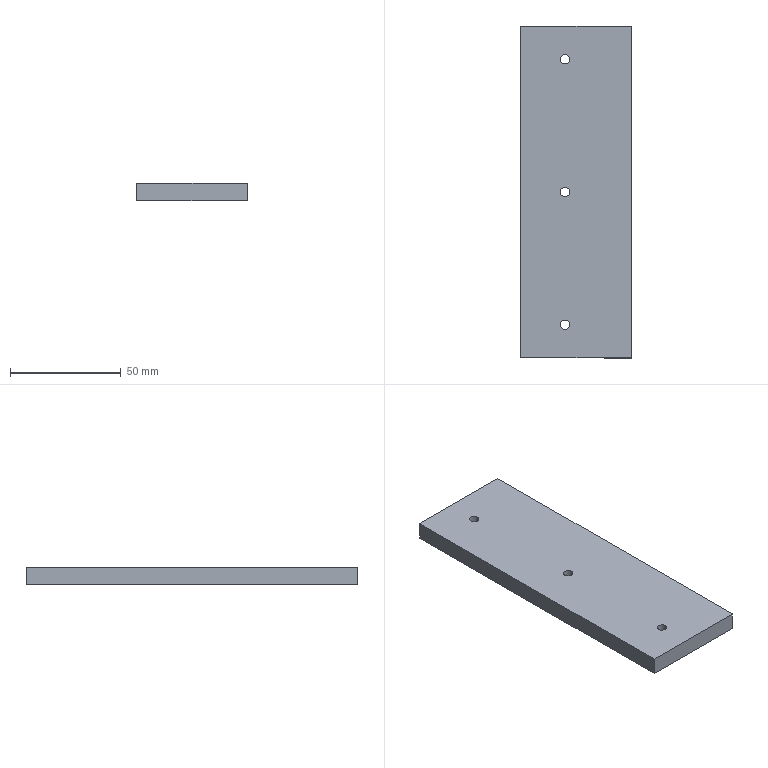Part | SolidWorks | features Chamfer 1, Extrusion 1, HoleWzd 1 | 1 solid | 12 faces | box 50 x 150 x 8 mm | volume 59667 mm3 | cylinder 6 | plane 6 | commonest cylinder face diameters 4.2 x6
STEP:
#1=CARTESIAN_POINT('',(-7.1,60.,-4.));
#2=VERTEX_POINT('',#1);
#3=CARTESIAN_POINT('',(-2.9,60.,-4.));
#4=VERTEX_POINT('',#3);
#5=CARTESIAN_POINT('',(-5.,60.,-4.));
#6=DIRECTION('',(0.,0.,1.));
#7=DIRECTION('',(1.,0.,0.));
#8=AXIS2_PLACEMENT_3D('',#5,#6,#7);
#9=CIRCLE('',#8,2.1);
#10=EDGE_CURVE('',#2,#4,#9,.T.);
#11=ORIENTED_EDGE('',*,*,#10,.F.);
#12=CARTESIAN_POINT('',(-7.1,60.,4.));
#13=VERTEX_POINT('',#12);
#14=CARTESIAN_POINT('',(-7.1,60.,4.));
#15=DIRECTION('',(0.,0.,1.));
#16=VECTOR('',#15,1000.);
#17=LINE('',#14,#16);
#18=EDGE_CURVE('',#2,#13,#17,.T.);
#19=ORIENTED_EDGE('',*,*,#18,.T.);
#20=CARTESIAN_POINT('',(-2.9,60.,4.));
#21=VERTEX_POINT('',#20);
#22=CARTESIAN_POINT('',(-5.,60.,4.));
#23=DIRECTION('',(0.,0.,1.));
#24=DIRECTION('',(1.,0.,0.));
#25=AXIS2_PLACEMENT_3D('',#22,#23,#24);
#26=CIRCLE('',#25,2.1);
#27=EDGE_CURVE('',#13,#21,#26,.T.);
#28=ORIENTED_EDGE('',*,*,#27,.T.);
#29=CARTESIAN_POINT('',(-2.9,60.,4.));
#30=DIRECTION('',(0.,0.,1.));
#31=VECTOR('',#30,1000.);
#32=LINE('',#29,#31);
#33=EDGE_CURVE('',#4,#21,#32,.T.);
#34=ORIENTED_EDGE('',*,*,#33,.F.);
#35=EDGE_LOOP('',(#11,#19,#28,#34));
#36=FACE_OUTER_BOUND('',#35,.T.);
#37=CARTESIAN_POINT('',(-5.,60.,4.));
#38=DIRECTION('',(0.,0.,1.));
#39=DIRECTION('',(1.,0.,0.));
#40=AXIS2_PLACEMENT_3D('',#37,#38,#39);
#41=CYLINDRICAL_SURFACE('',#40,2.1);
#42=ADVANCED_FACE('',(#36),#41,.F.);
#43=CARTESIAN_POINT('',(-7.1,-60.,-4.));
#44=VERTEX_POINT('',#43);
#45=CARTESIAN_POINT('',(-2.9,-60.,-4.));
#46=VERTEX_POINT('',#45);
#47=CARTESIAN_POINT('',(-5.,-60.,-4.));
#48=DIRECTION('',(0.,0.,1.));
#49=DIRECTION('',(1.,0.,0.));
#50=AXIS2_PLACEMENT_3D('',#47,#48,#49);
#51=CIRCLE('',#50,2.1);
#52=EDGE_CURVE('',#44,#46,#51,.T.);
#53=ORIENTED_EDGE('',*,*,#52,.F.);
#54=CARTESIAN_POINT('',(-7.1,-60.,4.));
#55=VERTEX_POINT('',#54);
#56=CARTESIAN_POINT('',(-7.1,-60.,4.));
#57=DIRECTION('',(0.,0.,1.));
#58=VECTOR('',#57,1000.);
#59=LINE('',#56,#58);
#60=EDGE_CURVE('',#44,#55,#59,.T.);
#61=ORIENTED_EDGE('',*,*,#60,.T.);
#62=CARTESIAN_POINT('',(-2.9,-60.,4.));
#63=VERTEX_POINT('',#62);
#64=CARTESIAN_POINT('',(-5.,-60.,4.));
#65=DIRECTION('',(0.,0.,1.));
#66=DIRECTION('',(1.,0.,0.));
#67=AXIS2_PLACEMENT_3D('',#64,#65,#66);
#68=CIRCLE('',#67,2.1);
#69=EDGE_CURVE('',#55,#63,#68,.T.);
#70=ORIENTED_EDGE('',*,*,#69,.T.);
#71=CARTESIAN_POINT('',(-2.9,-60.,4.));
#72=DIRECTION('',(0.,0.,1.));
#73=VECTOR('',#72,1000.);
#74=LINE('',#71,#73);
#75=EDGE_CURVE('',#46,#63,#74,.T.);
#76=ORIENTED_EDGE('',*,*,#75,.F.);
#77=EDGE_LOOP('',(#53,#61,#70,#76));
#78=FACE_OUTER_BOUND('',#77,.T.);
#79=CARTESIAN_POINT('',(-5.,-60.,4.));
#80=DIRECTION('',(0.,0.,1.));
#81=DIRECTION('',(1.,0.,0.));
#82=AXIS2_PLACEMENT_3D('',#79,#80,#81);
#83=CYLINDRICAL_SURFACE('',#82,2.1);
#84=ADVANCED_FACE('',(#78),#83,.F.);
#85=CARTESIAN_POINT('',(-7.1,0.,-4.));
#86=VERTEX_POINT('',#85);
#87=CARTESIAN_POINT('',(-2.9,0.,-4.));
#88=VERTEX_POINT('',#87);
#89=CARTESIAN_POINT('',(-5.,0.,-4.));
#90=DIRECTION('',(0.,0.,1.));
#91=DIRECTION('',(1.,0.,0.));
#92=AXIS2_PLACEMENT_3D('',#89,#90,#91);
#93=CIRCLE('',#92,2.1);
#94=EDGE_CURVE('',#86,#88,#93,.T.);
#95=ORIENTED_EDGE('',*,*,#94,.F.);
#96=CARTESIAN_POINT('',(-7.1,0.,4.));
#97=VERTEX_POINT('',#96);
#98=CARTESIAN_POINT('',(-7.1,0.,4.));
#99=DIRECTION('',(0.,0.,1.));
#100=VECTOR('',#99,1000.);
#101=LINE('',#98,#100);
#102=EDGE_CURVE('',#86,#97,#101,.T.);
#103=ORIENTED_EDGE('',*,*,#102,.T.);
#104=CARTESIAN_POINT('',(-2.9,0.,4.));
#105=VERTEX_POINT('',#104);
#106=CARTESIAN_POINT('',(-5.,0.,4.));
#107=DIRECTION('',(0.,0.,1.));
#108=DIRECTION('',(1.,0.,0.));
#109=AXIS2_PLACEMENT_3D('',#106,#107,#108);
#110=CIRCLE('',#109,2.1);
#111=EDGE_CURVE('',#97,#105,#110,.T.);
#112=ORIENTED_EDGE('',*,*,#111,.T.);
#113=CARTESIAN_POINT('',(-2.9,0.,4.));
#114=DIRECTION('',(0.,0.,1.));
#115=VECTOR('',#114,1000.);
#116=LINE('',#113,#115);
#117=EDGE_CURVE('',#88,#105,#116,.T.);
#118=ORIENTED_EDGE('',*,*,#117,.F.);
#119=EDGE_LOOP('',(#95,#103,#112,#118));
#120=FACE_OUTER_BOUND('',#119,.T.);
#121=CARTESIAN_POINT('',(-5.,0.,4.));
#122=DIRECTION('',(0.,0.,1.));
#123=DIRECTION('',(1.,0.,0.));
#124=AXIS2_PLACEMENT_3D('',#121,#122,#123);
#125=CYLINDRICAL_SURFACE('',#124,2.1);
#126=ADVANCED_FACE('',(#120),#125,.F.);
#127=CARTESIAN_POINT('',(-25.,75.,-4.));
#128=VERTEX_POINT('',#127);
#129=CARTESIAN_POINT('',(-25.,-75.,-4.));
#130=VERTEX_POINT('',#129);
#131=CARTESIAN_POINT('',(-25.,-75.,-4.));
#132=DIRECTION('',(0.,-1.,0.));
#133=VECTOR('',#132,1000.);
#134=LINE('',#131,#133);
#135=EDGE_CURVE('',#128,#130,#134,.T.);
#136=ORIENTED_EDGE('',*,*,#135,.T.);
#137=CARTESIAN_POINT('',(-25.,-75.,4.));
#138=VERTEX_POINT('',#137);
#139=CARTESIAN_POINT('',(-25.,-75.,4.));
#140=DIRECTION('',(0.,0.,-1.));
#141=VECTOR('',#140,1000.);
#142=LINE('',#139,#141);
#143=EDGE_CURVE('',#138,#130,#142,.T.);
#144=ORIENTED_EDGE('',*,*,#143,.F.);
#145=CARTESIAN_POINT('',(-25.,75.,4.));
#146=VERTEX_POINT('',#145);
#147=CARTESIAN_POINT('',(-25.,-75.,4.));
#148=DIRECTION('',(0.,-1.,0.));
#149=VECTOR('',#148,1000.);
#150=LINE('',#147,#149);
#151=EDGE_CURVE('',#146,#138,#150,.T.);
#152=ORIENTED_EDGE('',*,*,#151,.F.);
#153=CARTESIAN_POINT('',(-25.,75.,4.));
#154=DIRECTION('',(0.,0.,-1.));
#155=VECTOR('',#154,1000.);
#156=LINE('',#153,#155);
#157=EDGE_CURVE('',#146,#128,#156,.T.);
#158=ORIENTED_EDGE('',*,*,#157,.T.);
#159=EDGE_LOOP('',(#136,#144,#152,#158));
#160=FACE_OUTER_BOUND('',#159,.T.);
#161=CARTESIAN_POINT('',(-25.,-75.,4.));
#162=DIRECTION('',(1.,0.,0.));
#163=DIRECTION('',(0.,0.,-1.));
#164=AXIS2_PLACEMENT_3D('',#161,#162,#163);
#165=PLANE('',#164);
#166=ADVANCED_FACE('',(#160),#165,.F.);
#167=CARTESIAN_POINT('',(25.,-75.,-4.));
#168=VERTEX_POINT('',#167);
#169=CARTESIAN_POINT('',(25.,-75.,-4.));
#170=DIRECTION('',(1.,0.,0.));
#171=VECTOR('',#170,1000.);
#172=LINE('',#169,#171);
#173=EDGE_CURVE('',#130,#168,#172,.T.);
#174=ORIENTED_EDGE('',*,*,#173,.T.);
#175=CARTESIAN_POINT('',(25.,-75.,4.));
#176=VERTEX_POINT('',#175);
#177=CARTESIAN_POINT('',(25.,-75.,4.));
#178=DIRECTION('',(0.,0.,-1.));
#179=VECTOR('',#178,1000.);
#180=LINE('',#177,#179);
#181=EDGE_CURVE('',#176,#168,#180,.T.);
#182=ORIENTED_EDGE('',*,*,#181,.F.);
#183=CARTESIAN_POINT('',(25.,-75.,4.));
#184=DIRECTION('',(1.,0.,0.));
#185=VECTOR('',#184,1000.);
#186=LINE('',#183,#185);
#187=EDGE_CURVE('',#138,#176,#186,.T.);
#188=ORIENTED_EDGE('',*,*,#187,.F.);
#189=ORIENTED_EDGE('',*,*,#143,.T.);
#190=EDGE_LOOP('',(#174,#182,#188,#189));
#191=FACE_OUTER_BOUND('',#190,.T.);
#192=CARTESIAN_POINT('',(25.,-75.,4.));
#193=DIRECTION('',(0.,1.,0.));
#194=DIRECTION('',(-1.,0.,0.));
#195=AXIS2_PLACEMENT_3D('',#192,#193,#194);
#196=PLANE('',#195);
#197=ADVANCED_FACE('',(#191),#196,.F.);
#198=CARTESIAN_POINT('',(25.,75.,-4.));
#199=VERTEX_POINT('',#198);
#200=CARTESIAN_POINT('',(25.,-75.,-4.));
#201=DIRECTION('',(0.,1.,0.));
#202=VECTOR('',#201,1000.);
#203=LINE('',#200,#202);
#204=EDGE_CURVE('',#168,#199,#203,.T.);
#205=ORIENTED_EDGE('',*,*,#204,.T.);
#206=CARTESIAN_POINT('',(25.,75.,4.));
#207=VERTEX_POINT('',#206);
#208=CARTESIAN_POINT('',(25.,75.,4.));
#209=DIRECTION('',(0.,0.,-1.));
#210=VECTOR('',#209,1000.);
#211=LINE('',#208,#210);
#212=EDGE_CURVE('',#207,#199,#211,.T.);
#213=ORIENTED_EDGE('',*,*,#212,.F.);
#214=CARTESIAN_POINT('',(25.,-75.,4.));
#215=DIRECTION('',(0.,1.,0.));
#216=VECTOR('',#215,1000.);
#217=LINE('',#214,#216);
#218=EDGE_CURVE('',#176,#207,#217,.T.);
#219=ORIENTED_EDGE('',*,*,#218,.F.);
#220=ORIENTED_EDGE('',*,*,#181,.T.);
#221=EDGE_LOOP('',(#205,#213,#219,#220));
#222=FACE_OUTER_BOUND('',#221,.T.);
#223=CARTESIAN_POINT('',(25.,-75.,4.));
#224=DIRECTION('',(-1.,0.,0.));
#225=DIRECTION('',(0.,0.,1.));
#226=AXIS2_PLACEMENT_3D('',#223,#224,#225);
#227=PLANE('',#226);
#228=ADVANCED_FACE('',(#222),#227,.F.);
#229=CARTESIAN_POINT('',(25.,75.,-4.));
#230=DIRECTION('',(-1.,0.,0.));
#231=VECTOR('',#230,1000.);
#232=LINE('',#229,#231);
#233=EDGE_CURVE('',#199,#128,#232,.T.);
#234=ORIENTED_EDGE('',*,*,#233,.T.);
#235=ORIENTED_EDGE('',*,*,#157,.F.);
#236=CARTESIAN_POINT('',(25.,75.,4.));
#237=DIRECTION('',(-1.,0.,0.));
#238=VECTOR('',#237,1000.);
#239=LINE('',#236,#238);
#240=EDGE_CURVE('',#207,#146,#239,.T.);
#241=ORIENTED_EDGE('',*,*,#240,.F.);
#242=ORIENTED_EDGE('',*,*,#212,.T.);
#243=EDGE_LOOP('',(#234,#235,#241,#242));
#244=FACE_OUTER_BOUND('',#243,.T.);
#245=CARTESIAN_POINT('',(25.,75.,4.));
#246=DIRECTION('',(0.,-1.,0.));
#247=DIRECTION('',(0.,0.,-1.));
#248=AXIS2_PLACEMENT_3D('',#245,#246,#247);
#249=PLANE('',#248);
#250=ADVANCED_FACE('',(#244),#249,.F.);
#251=CARTESIAN_POINT('',(-5.,60.,4.));
#252=DIRECTION('',(0.,0.,1.));
#253=DIRECTION('',(1.,0.,0.));
#254=AXIS2_PLACEMENT_3D('',#251,#252,#253);
#255=CIRCLE('',#254,2.1);
#256=EDGE_CURVE('',#21,#13,#255,.T.);
#257=ORIENTED_EDGE('',*,*,#256,.F.);
#258=ORIENTED_EDGE('',*,*,#27,.F.);
#259=EDGE_LOOP('',(#257,#258));
#260=FACE_BOUND('',#259,.T.);
#261=CARTESIAN_POINT('',(-5.,-60.,4.));
#262=DIRECTION('',(0.,0.,1.));
#263=DIRECTION('',(1.,0.,0.));
#264=AXIS2_PLACEMENT_3D('',#261,#262,#263);
#265=CIRCLE('',#264,2.1);
#266=EDGE_CURVE('',#63,#55,#265,.T.);
#267=ORIENTED_EDGE('',*,*,#266,.F.);
#268=ORIENTED_EDGE('',*,*,#69,.F.);
#269=EDGE_LOOP('',(#267,#268));
#270=FACE_BOUND('',#269,.T.);
#271=CARTESIAN_POINT('',(-5.,0.,4.));
#272=DIRECTION('',(0.,0.,1.));
#273=DIRECTION('',(1.,0.,0.));
#274=AXIS2_PLACEMENT_3D('',#271,#272,#273);
#275=CIRCLE('',#274,2.1);
#276=EDGE_CURVE('',#105,#97,#275,.T.);
#277=ORIENTED_EDGE('',*,*,#276,.F.);
#278=ORIENTED_EDGE('',*,*,#111,.F.);
#279=EDGE_LOOP('',(#277,#278));
#280=FACE_BOUND('',#279,.T.);
#281=ORIENTED_EDGE('',*,*,#151,.T.);
#282=ORIENTED_EDGE('',*,*,#187,.T.);
#283=ORIENTED_EDGE('',*,*,#218,.T.);
#284=ORIENTED_EDGE('',*,*,#240,.T.);
#285=EDGE_LOOP('',(#281,#282,#283,#284));
#286=FACE_OUTER_BOUND('',#285,.T.);
#287=CARTESIAN_POINT('',(0.,0.,4.));
#288=DIRECTION('',(0.,0.,1.));
#289=DIRECTION('',(1.,0.,0.));
#290=AXIS2_PLACEMENT_3D('',#287,#288,#289);
#291=PLANE('',#290);
#292=ADVANCED_FACE('',(#260,#270,#280,#286),#291,.T.);
#293=CARTESIAN_POINT('',(-5.,60.,-4.));
#294=DIRECTION('',(0.,0.,1.));
#295=DIRECTION('',(1.,0.,0.));
#296=AXIS2_PLACEMENT_3D('',#293,#294,#295);
#297=CIRCLE('',#296,2.1);
#298=EDGE_CURVE('',#4,#2,#297,.T.);
#299=ORIENTED_EDGE('',*,*,#298,.T.);
#300=ORIENTED_EDGE('',*,*,#10,.T.);
#301=EDGE_LOOP('',(#299,#300));
#302=FACE_BOUND('',#301,.T.);
#303=CARTESIAN_POINT('',(-5.,-60.,-4.));
#304=DIRECTION('',(0.,0.,1.));
#305=DIRECTION('',(1.,0.,0.));
#306=AXIS2_PLACEMENT_3D('',#303,#304,#305);
#307=CIRCLE('',#306,2.1);
#308=EDGE_CURVE('',#46,#44,#307,.T.);
#309=ORIENTED_EDGE('',*,*,#308,.T.);
#310=ORIENTED_EDGE('',*,*,#52,.T.);
#311=EDGE_LOOP('',(#309,#310));
#312=FACE_BOUND('',#311,.T.);
#313=CARTESIAN_POINT('',(-5.,0.,-4.));
#314=DIRECTION('',(0.,0.,1.));
#315=DIRECTION('',(1.,0.,0.));
#316=AXIS2_PLACEMENT_3D('',#313,#314,#315);
#317=CIRCLE('',#316,2.1);
#318=EDGE_CURVE('',#88,#86,#317,.T.);
#319=ORIENTED_EDGE('',*,*,#318,.T.);
#320=ORIENTED_EDGE('',*,*,#94,.T.);
#321=EDGE_LOOP('',(#319,#320));
#322=FACE_BOUND('',#321,.T.);
#323=ORIENTED_EDGE('',*,*,#135,.F.);
#324=ORIENTED_EDGE('',*,*,#233,.F.);
#325=ORIENTED_EDGE('',*,*,#204,.F.);
#326=ORIENTED_EDGE('',*,*,#173,.F.);
#327=EDGE_LOOP('',(#323,#324,#325,#326));
#328=FACE_OUTER_BOUND('',#327,.T.);
#329=CARTESIAN_POINT('',(0.,0.,-4.));
#330=DIRECTION('',(0.,0.,1.));
#331=DIRECTION('',(1.,0.,0.));
#332=AXIS2_PLACEMENT_3D('',#329,#330,#331);
#333=PLANE('',#332);
#334=ADVANCED_FACE('',(#302,#312,#322,#328),#333,.F.);
#335=ORIENTED_EDGE('',*,*,#102,.F.);
#336=ORIENTED_EDGE('',*,*,#318,.F.);
#337=ORIENTED_EDGE('',*,*,#117,.T.);
#338=ORIENTED_EDGE('',*,*,#276,.T.);
#339=EDGE_LOOP('',(#335,#336,#337,#338));
#340=FACE_OUTER_BOUND('',#339,.T.);
#341=CARTESIAN_POINT('',(-5.,0.,4.));
#342=DIRECTION('',(0.,0.,1.));
#343=DIRECTION('',(1.,0.,0.));
#344=AXIS2_PLACEMENT_3D('',#341,#342,#343);
#345=CYLINDRICAL_SURFACE('',#344,2.1);
#346=ADVANCED_FACE('',(#340),#345,.F.);
#347=ORIENTED_EDGE('',*,*,#60,.F.);
#348=ORIENTED_EDGE('',*,*,#308,.F.);
#349=ORIENTED_EDGE('',*,*,#75,.T.);
#350=ORIENTED_EDGE('',*,*,#266,.T.);
#351=EDGE_LOOP('',(#347,#348,#349,#350));
#352=FACE_OUTER_BOUND('',#351,.T.);
#353=CARTESIAN_POINT('',(-5.,-60.,4.));
#354=DIRECTION('',(0.,0.,1.));
#355=DIRECTION('',(1.,0.,0.));
#356=AXIS2_PLACEMENT_3D('',#353,#354,#355);
#357=CYLINDRICAL_SURFACE('',#356,2.1);
#358=ADVANCED_FACE('',(#352),#357,.F.);
#359=ORIENTED_EDGE('',*,*,#18,.F.);
#360=ORIENTED_EDGE('',*,*,#298,.F.);
#361=ORIENTED_EDGE('',*,*,#33,.T.);
#362=ORIENTED_EDGE('',*,*,#256,.T.);
#363=EDGE_LOOP('',(#359,#360,#361,#362));
#364=FACE_OUTER_BOUND('',#363,.T.);
#365=CARTESIAN_POINT('',(-5.,60.,4.));
#366=DIRECTION('',(0.,0.,1.));
#367=DIRECTION('',(1.,0.,0.));
#368=AXIS2_PLACEMENT_3D('',#365,#366,#367);
#369=CYLINDRICAL_SURFACE('',#368,2.1);
#370=ADVANCED_FACE('',(#364),#369,.F.);
#371=CLOSED_SHELL('',(#42,#84,#126,#166,#197,#228,#250,#292,#334,#346,#358,#370));
#372=MANIFOLD_SOLID_BREP('',#371);
#373=CARTESIAN_POINT('',(0.,0.,0.));
#374=DIRECTION('',(0.,0.,1.));
#375=DIRECTION('',(1.,0.,0.));
#376=AXIS2_PLACEMENT_3D('',#373,#374,#375);
#377=(LENGTH_UNIT()NAMED_UNIT(*)SI_UNIT(.MILLI.,.METRE.));
#378=UNCERTAINTY_MEASURE_WITH_UNIT(LENGTH_MEASURE(0.00001),#377,'','');
#379=(NAMED_UNIT(*)PLANE_ANGLE_UNIT()SI_UNIT($,.RADIAN.));
#380=(NAMED_UNIT(*)SI_UNIT($,.STERADIAN.)SOLID_ANGLE_UNIT());
#381=(GEOMETRIC_REPRESENTATION_CONTEXT(3)GLOBAL_UNCERTAINTY_ASSIGNED_CONTEXT((#378))GLOBAL_UNIT_ASSIGNED_CONTEXT((#377,#379,#380))REPRESENTATION_CONTEXT('',''));
#382=ADVANCED_BREP_SHAPE_REPRESENTATION('',(#372,#376),#381);